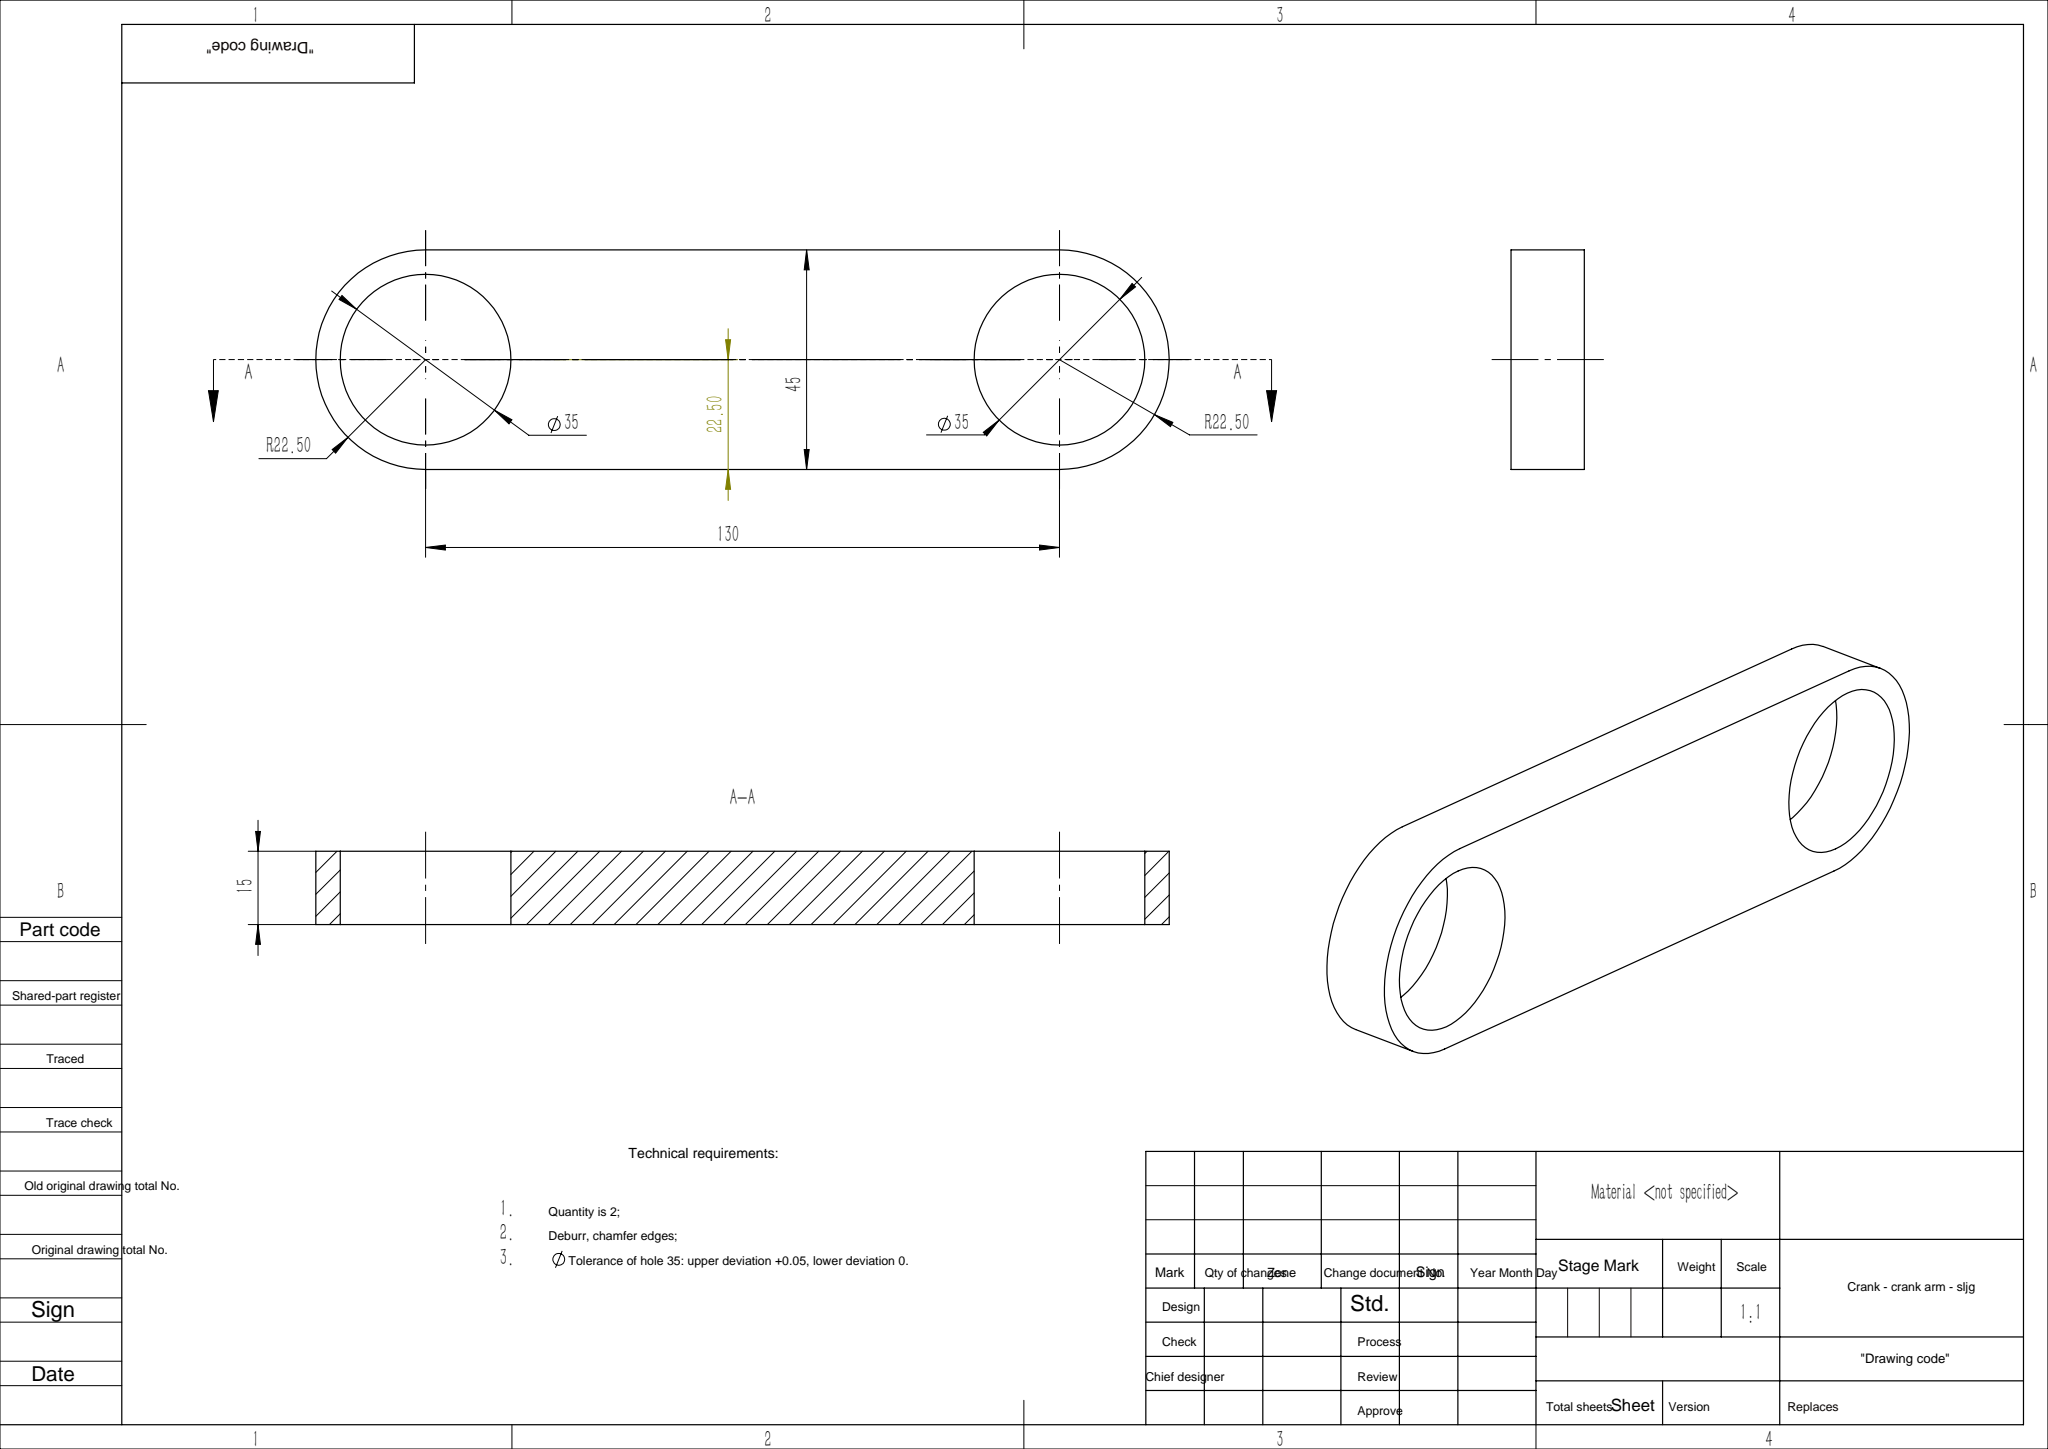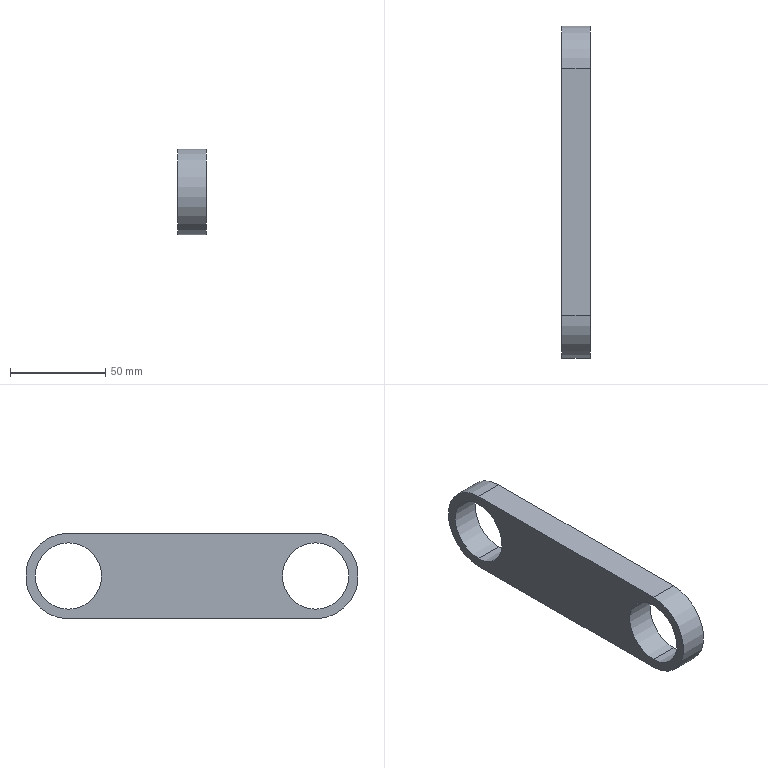Part | SolidWorks | features ICE 2, Extrusion 1 | 1 solid | 10 faces | box 15 x 175 x 45 mm | volume 82743 mm3 | cylinder 6 | plane 4 | commonest cylinder face diameters 35 x4 45 x2
STEP:
#1=CARTESIAN_POINT('',(15.,-130.,-17.5));
#2=VERTEX_POINT('',#1);
#3=CARTESIAN_POINT('',(15.,-130.,17.5));
#4=VERTEX_POINT('',#3);
#5=CARTESIAN_POINT('',(15.,-130.,0.));
#6=DIRECTION('',(-1.,0.,0.));
#7=DIRECTION('',(0.,0.,1.));
#8=AXIS2_PLACEMENT_3D('',#5,#6,#7);
#9=CIRCLE('',#8,17.5);
#10=EDGE_CURVE('',#2,#4,#9,.T.);
#11=ORIENTED_EDGE('',*,*,#10,.F.);
#12=CARTESIAN_POINT('',(0.,-130.,-17.5));
#13=VERTEX_POINT('',#12);
#14=CARTESIAN_POINT('',(15.,-130.,-17.5));
#15=DIRECTION('',(-1.,0.,0.));
#16=VECTOR('',#15,1000.);
#17=LINE('',#14,#16);
#18=EDGE_CURVE('',#2,#13,#17,.T.);
#19=ORIENTED_EDGE('',*,*,#18,.T.);
#20=CARTESIAN_POINT('',(0.,-130.,17.5));
#21=VERTEX_POINT('',#20);
#22=CARTESIAN_POINT('',(0.,-130.,0.));
#23=DIRECTION('',(-1.,0.,0.));
#24=DIRECTION('',(0.,0.,1.));
#25=AXIS2_PLACEMENT_3D('',#22,#23,#24);
#26=CIRCLE('',#25,17.5);
#27=EDGE_CURVE('',#13,#21,#26,.T.);
#28=ORIENTED_EDGE('',*,*,#27,.T.);
#29=CARTESIAN_POINT('',(15.,-130.,17.5));
#30=DIRECTION('',(-1.,0.,0.));
#31=VECTOR('',#30,1000.);
#32=LINE('',#29,#31);
#33=EDGE_CURVE('',#4,#21,#32,.T.);
#34=ORIENTED_EDGE('',*,*,#33,.F.);
#35=EDGE_LOOP('',(#11,#19,#28,#34));
#36=FACE_OUTER_BOUND('',#35,.T.);
#37=CARTESIAN_POINT('',(15.,-130.,0.));
#38=DIRECTION('',(-1.,0.,0.));
#39=DIRECTION('',(0.,0.,1.));
#40=AXIS2_PLACEMENT_3D('',#37,#38,#39);
#41=CYLINDRICAL_SURFACE('',#40,17.5);
#42=ADVANCED_FACE('',(#36),#41,.F.);
#43=CARTESIAN_POINT('',(0.,0.,17.5));
#44=VERTEX_POINT('',#43);
#45=CARTESIAN_POINT('',(0.,0.,-17.5));
#46=VERTEX_POINT('',#45);
#47=CARTESIAN_POINT('',(0.,0.,0.));
#48=DIRECTION('',(1.,0.,0.));
#49=DIRECTION('',(0.,0.,-1.));
#50=AXIS2_PLACEMENT_3D('',#47,#48,#49);
#51=CIRCLE('',#50,17.5);
#52=EDGE_CURVE('',#44,#46,#51,.T.);
#53=ORIENTED_EDGE('',*,*,#52,.F.);
#54=CARTESIAN_POINT('',(15.,0.,17.5));
#55=VERTEX_POINT('',#54);
#56=CARTESIAN_POINT('',(0.,0.,17.5));
#57=DIRECTION('',(1.,0.,0.));
#58=VECTOR('',#57,1000.);
#59=LINE('',#56,#58);
#60=EDGE_CURVE('',#44,#55,#59,.T.);
#61=ORIENTED_EDGE('',*,*,#60,.T.);
#62=CARTESIAN_POINT('',(15.,0.,-17.5));
#63=VERTEX_POINT('',#62);
#64=CARTESIAN_POINT('',(15.,0.,0.));
#65=DIRECTION('',(1.,0.,0.));
#66=DIRECTION('',(0.,0.,-1.));
#67=AXIS2_PLACEMENT_3D('',#64,#65,#66);
#68=CIRCLE('',#67,17.5);
#69=EDGE_CURVE('',#55,#63,#68,.T.);
#70=ORIENTED_EDGE('',*,*,#69,.T.);
#71=CARTESIAN_POINT('',(0.,0.,-17.5));
#72=DIRECTION('',(1.,0.,0.));
#73=VECTOR('',#72,1000.);
#74=LINE('',#71,#73);
#75=EDGE_CURVE('',#46,#63,#74,.T.);
#76=ORIENTED_EDGE('',*,*,#75,.F.);
#77=EDGE_LOOP('',(#53,#61,#70,#76));
#78=FACE_OUTER_BOUND('',#77,.T.);
#79=CARTESIAN_POINT('',(0.,0.,0.));
#80=DIRECTION('',(1.,0.,0.));
#81=DIRECTION('',(0.,0.,-1.));
#82=AXIS2_PLACEMENT_3D('',#79,#80,#81);
#83=CYLINDRICAL_SURFACE('',#82,17.5);
#84=ADVANCED_FACE('',(#78),#83,.F.);
#85=CARTESIAN_POINT('',(0.,0.,-22.5));
#86=VERTEX_POINT('',#85);
#87=CARTESIAN_POINT('',(0.,-130.,-22.5));
#88=VERTEX_POINT('',#87);
#89=CARTESIAN_POINT('',(0.,0.,-22.5));
#90=DIRECTION('',(0.,-1.,0.));
#91=VECTOR('',#90,1000.);
#92=LINE('',#89,#91);
#93=EDGE_CURVE('',#86,#88,#92,.T.);
#94=ORIENTED_EDGE('',*,*,#93,.F.);
#95=CARTESIAN_POINT('',(15.,0.,-22.5));
#96=VERTEX_POINT('',#95);
#97=CARTESIAN_POINT('',(15.,0.,-22.5));
#98=DIRECTION('',(-1.,0.,0.));
#99=VECTOR('',#98,1000.);
#100=LINE('',#97,#99);
#101=EDGE_CURVE('',#96,#86,#100,.T.);
#102=ORIENTED_EDGE('',*,*,#101,.F.);
#103=CARTESIAN_POINT('',(15.,-130.,-22.5));
#104=VERTEX_POINT('',#103);
#105=CARTESIAN_POINT('',(15.,0.,-22.5));
#106=DIRECTION('',(0.,-1.,0.));
#107=VECTOR('',#106,1000.);
#108=LINE('',#105,#107);
#109=EDGE_CURVE('',#96,#104,#108,.T.);
#110=ORIENTED_EDGE('',*,*,#109,.T.);
#111=CARTESIAN_POINT('',(15.,-130.,-22.5));
#112=DIRECTION('',(-1.,0.,0.));
#113=VECTOR('',#112,1000.);
#114=LINE('',#111,#113);
#115=EDGE_CURVE('',#104,#88,#114,.T.);
#116=ORIENTED_EDGE('',*,*,#115,.T.);
#117=EDGE_LOOP('',(#94,#102,#110,#116));
#118=FACE_OUTER_BOUND('',#117,.T.);
#119=CARTESIAN_POINT('',(15.,0.,-22.5));
#120=DIRECTION('',(0.,0.,-1.));
#121=DIRECTION('',(0.,1.,0.));
#122=AXIS2_PLACEMENT_3D('',#119,#120,#121);
#123=PLANE('',#122);
#124=ADVANCED_FACE('',(#118),#123,.T.);
#125=CARTESIAN_POINT('',(0.,0.,22.5));
#126=VERTEX_POINT('',#125);
#127=CARTESIAN_POINT('',(0.,0.,0.));
#128=DIRECTION('',(1.,0.,0.));
#129=DIRECTION('',(0.,0.,-1.));
#130=AXIS2_PLACEMENT_3D('',#127,#128,#129);
#131=CIRCLE('',#130,22.5);
#132=EDGE_CURVE('',#86,#126,#131,.T.);
#133=ORIENTED_EDGE('',*,*,#132,.T.);
#134=CARTESIAN_POINT('',(15.,0.,22.5));
#135=VERTEX_POINT('',#134);
#136=CARTESIAN_POINT('',(15.,0.,22.5));
#137=DIRECTION('',(-1.,0.,0.));
#138=VECTOR('',#137,1000.);
#139=LINE('',#136,#138);
#140=EDGE_CURVE('',#135,#126,#139,.T.);
#141=ORIENTED_EDGE('',*,*,#140,.F.);
#142=CARTESIAN_POINT('',(15.,0.,0.));
#143=DIRECTION('',(1.,0.,0.));
#144=DIRECTION('',(0.,0.,-1.));
#145=AXIS2_PLACEMENT_3D('',#142,#143,#144);
#146=CIRCLE('',#145,22.5);
#147=EDGE_CURVE('',#96,#135,#146,.T.);
#148=ORIENTED_EDGE('',*,*,#147,.F.);
#149=ORIENTED_EDGE('',*,*,#101,.T.);
#150=EDGE_LOOP('',(#133,#141,#148,#149));
#151=FACE_OUTER_BOUND('',#150,.T.);
#152=CARTESIAN_POINT('',(15.,0.,0.));
#153=DIRECTION('',(-1.,0.,0.));
#154=DIRECTION('',(0.,0.,1.));
#155=AXIS2_PLACEMENT_3D('',#152,#153,#154);
#156=CYLINDRICAL_SURFACE('',#155,22.5);
#157=ADVANCED_FACE('',(#151),#156,.T.);
#158=CARTESIAN_POINT('',(0.,-130.,22.5));
#159=VERTEX_POINT('',#158);
#160=CARTESIAN_POINT('',(0.,0.,22.5));
#161=DIRECTION('',(0.,-1.,0.));
#162=VECTOR('',#161,1000.);
#163=LINE('',#160,#162);
#164=EDGE_CURVE('',#126,#159,#163,.T.);
#165=ORIENTED_EDGE('',*,*,#164,.T.);
#166=CARTESIAN_POINT('',(15.,-130.,22.5));
#167=VERTEX_POINT('',#166);
#168=CARTESIAN_POINT('',(15.,-130.,22.5));
#169=DIRECTION('',(-1.,0.,0.));
#170=VECTOR('',#169,1000.);
#171=LINE('',#168,#170);
#172=EDGE_CURVE('',#167,#159,#171,.T.);
#173=ORIENTED_EDGE('',*,*,#172,.F.);
#174=CARTESIAN_POINT('',(15.,0.,22.5));
#175=DIRECTION('',(0.,-1.,0.));
#176=VECTOR('',#175,1000.);
#177=LINE('',#174,#176);
#178=EDGE_CURVE('',#135,#167,#177,.T.);
#179=ORIENTED_EDGE('',*,*,#178,.F.);
#180=ORIENTED_EDGE('',*,*,#140,.T.);
#181=EDGE_LOOP('',(#165,#173,#179,#180));
#182=FACE_OUTER_BOUND('',#181,.T.);
#183=CARTESIAN_POINT('',(15.,0.,22.5));
#184=DIRECTION('',(0.,0.,-1.));
#185=DIRECTION('',(0.,1.,0.));
#186=AXIS2_PLACEMENT_3D('',#183,#184,#185);
#187=PLANE('',#186);
#188=ADVANCED_FACE('',(#182),#187,.F.);
#189=CARTESIAN_POINT('',(0.,-130.,0.));
#190=DIRECTION('',(1.,0.,0.));
#191=DIRECTION('',(0.,0.,-1.));
#192=AXIS2_PLACEMENT_3D('',#189,#190,#191);
#193=CIRCLE('',#192,22.5);
#194=EDGE_CURVE('',#159,#88,#193,.T.);
#195=ORIENTED_EDGE('',*,*,#194,.T.);
#196=ORIENTED_EDGE('',*,*,#115,.F.);
#197=CARTESIAN_POINT('',(15.,-130.,0.));
#198=DIRECTION('',(1.,0.,0.));
#199=DIRECTION('',(0.,0.,-1.));
#200=AXIS2_PLACEMENT_3D('',#197,#198,#199);
#201=CIRCLE('',#200,22.5);
#202=EDGE_CURVE('',#167,#104,#201,.T.);
#203=ORIENTED_EDGE('',*,*,#202,.F.);
#204=ORIENTED_EDGE('',*,*,#172,.T.);
#205=EDGE_LOOP('',(#195,#196,#203,#204));
#206=FACE_OUTER_BOUND('',#205,.T.);
#207=CARTESIAN_POINT('',(15.,-130.,0.));
#208=DIRECTION('',(-1.,0.,0.));
#209=DIRECTION('',(0.,0.,1.));
#210=AXIS2_PLACEMENT_3D('',#207,#208,#209);
#211=CYLINDRICAL_SURFACE('',#210,22.5);
#212=ADVANCED_FACE('',(#206),#211,.T.);
#213=CARTESIAN_POINT('',(15.,-130.,0.));
#214=DIRECTION('',(-1.,0.,0.));
#215=DIRECTION('',(0.,0.,1.));
#216=AXIS2_PLACEMENT_3D('',#213,#214,#215);
#217=CIRCLE('',#216,17.5);
#218=EDGE_CURVE('',#4,#2,#217,.T.);
#219=ORIENTED_EDGE('',*,*,#218,.T.);
#220=ORIENTED_EDGE('',*,*,#10,.T.);
#221=EDGE_LOOP('',(#219,#220));
#222=FACE_BOUND('',#221,.T.);
#223=CARTESIAN_POINT('',(15.,0.,0.));
#224=DIRECTION('',(1.,0.,0.));
#225=DIRECTION('',(0.,0.,-1.));
#226=AXIS2_PLACEMENT_3D('',#223,#224,#225);
#227=CIRCLE('',#226,17.5);
#228=EDGE_CURVE('',#63,#55,#227,.T.);
#229=ORIENTED_EDGE('',*,*,#228,.F.);
#230=ORIENTED_EDGE('',*,*,#69,.F.);
#231=EDGE_LOOP('',(#229,#230));
#232=FACE_BOUND('',#231,.T.);
#233=ORIENTED_EDGE('',*,*,#109,.F.);
#234=ORIENTED_EDGE('',*,*,#147,.T.);
#235=ORIENTED_EDGE('',*,*,#178,.T.);
#236=ORIENTED_EDGE('',*,*,#202,.T.);
#237=EDGE_LOOP('',(#233,#234,#235,#236));
#238=FACE_OUTER_BOUND('',#237,.T.);
#239=CARTESIAN_POINT('',(15.,-130.,0.));
#240=DIRECTION('',(1.,0.,0.));
#241=DIRECTION('',(0.,0.,-1.));
#242=AXIS2_PLACEMENT_3D('',#239,#240,#241);
#243=PLANE('',#242);
#244=ADVANCED_FACE('',(#222,#232,#238),#243,.T.);
#245=CARTESIAN_POINT('',(0.,-130.,0.));
#246=DIRECTION('',(-1.,0.,0.));
#247=DIRECTION('',(0.,0.,1.));
#248=AXIS2_PLACEMENT_3D('',#245,#246,#247);
#249=CIRCLE('',#248,17.5);
#250=EDGE_CURVE('',#21,#13,#249,.T.);
#251=ORIENTED_EDGE('',*,*,#250,.F.);
#252=ORIENTED_EDGE('',*,*,#27,.F.);
#253=EDGE_LOOP('',(#251,#252));
#254=FACE_BOUND('',#253,.T.);
#255=CARTESIAN_POINT('',(0.,0.,0.));
#256=DIRECTION('',(1.,0.,0.));
#257=DIRECTION('',(0.,0.,-1.));
#258=AXIS2_PLACEMENT_3D('',#255,#256,#257);
#259=CIRCLE('',#258,17.5);
#260=EDGE_CURVE('',#46,#44,#259,.T.);
#261=ORIENTED_EDGE('',*,*,#260,.T.);
#262=ORIENTED_EDGE('',*,*,#52,.T.);
#263=EDGE_LOOP('',(#261,#262));
#264=FACE_BOUND('',#263,.T.);
#265=ORIENTED_EDGE('',*,*,#93,.T.);
#266=ORIENTED_EDGE('',*,*,#194,.F.);
#267=ORIENTED_EDGE('',*,*,#164,.F.);
#268=ORIENTED_EDGE('',*,*,#132,.F.);
#269=EDGE_LOOP('',(#265,#266,#267,#268));
#270=FACE_OUTER_BOUND('',#269,.T.);
#271=CARTESIAN_POINT('',(0.,-130.,0.));
#272=DIRECTION('',(1.,0.,0.));
#273=DIRECTION('',(0.,0.,-1.));
#274=AXIS2_PLACEMENT_3D('',#271,#272,#273);
#275=PLANE('',#274);
#276=ADVANCED_FACE('',(#254,#264,#270),#275,.F.);
#277=ORIENTED_EDGE('',*,*,#60,.F.);
#278=ORIENTED_EDGE('',*,*,#260,.F.);
#279=ORIENTED_EDGE('',*,*,#75,.T.);
#280=ORIENTED_EDGE('',*,*,#228,.T.);
#281=EDGE_LOOP('',(#277,#278,#279,#280));
#282=FACE_OUTER_BOUND('',#281,.T.);
#283=CARTESIAN_POINT('',(0.,0.,0.));
#284=DIRECTION('',(1.,0.,0.));
#285=DIRECTION('',(0.,0.,-1.));
#286=AXIS2_PLACEMENT_3D('',#283,#284,#285);
#287=CYLINDRICAL_SURFACE('',#286,17.5);
#288=ADVANCED_FACE('',(#282),#287,.F.);
#289=ORIENTED_EDGE('',*,*,#18,.F.);
#290=ORIENTED_EDGE('',*,*,#218,.F.);
#291=ORIENTED_EDGE('',*,*,#33,.T.);
#292=ORIENTED_EDGE('',*,*,#250,.T.);
#293=EDGE_LOOP('',(#289,#290,#291,#292));
#294=FACE_OUTER_BOUND('',#293,.T.);
#295=CARTESIAN_POINT('',(15.,-130.,0.));
#296=DIRECTION('',(-1.,0.,0.));
#297=DIRECTION('',(0.,0.,1.));
#298=AXIS2_PLACEMENT_3D('',#295,#296,#297);
#299=CYLINDRICAL_SURFACE('',#298,17.5);
#300=ADVANCED_FACE('',(#294),#299,.F.);
#301=CLOSED_SHELL('',(#42,#84,#124,#157,#188,#212,#244,#276,#288,#300));
#302=MANIFOLD_SOLID_BREP('',#301);
#303=CARTESIAN_POINT('',(0.,0.,0.));
#304=DIRECTION('',(0.,0.,1.));
#305=DIRECTION('',(1.,0.,0.));
#306=AXIS2_PLACEMENT_3D('',#303,#304,#305);
#307=(LENGTH_UNIT()NAMED_UNIT(*)SI_UNIT(.MILLI.,.METRE.));
#308=UNCERTAINTY_MEASURE_WITH_UNIT(LENGTH_MEASURE(0.00001),#307,'','');
#309=(NAMED_UNIT(*)PLANE_ANGLE_UNIT()SI_UNIT($,.RADIAN.));
#310=(NAMED_UNIT(*)SI_UNIT($,.STERADIAN.)SOLID_ANGLE_UNIT());
#311=(GEOMETRIC_REPRESENTATION_CONTEXT(3)GLOBAL_UNCERTAINTY_ASSIGNED_CONTEXT((#308))GLOBAL_UNIT_ASSIGNED_CONTEXT((#307,#309,#310))REPRESENTATION_CONTEXT('',''));
#312=ADVANCED_BREP_SHAPE_REPRESENTATION('',(#302,#306),#311);